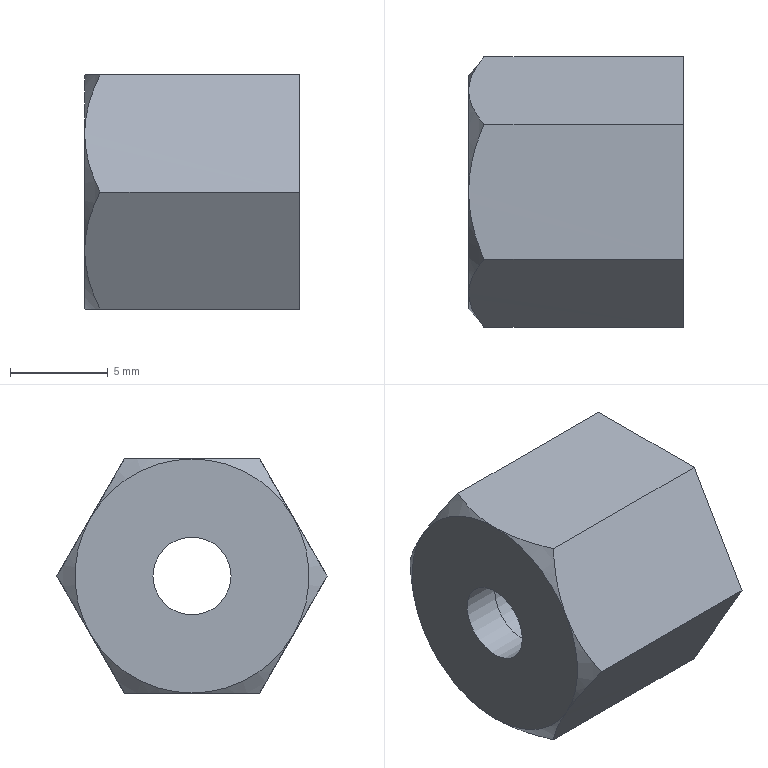Part | STEP file | 1-75.5 | 2 solids | 21 faces | box 11 x 13.856 x 12 mm | volume 966.779 mm3 | plane 11 | cone 6 | cylinder 4 | commonest cylinder face diameters 4 x2 8 x2